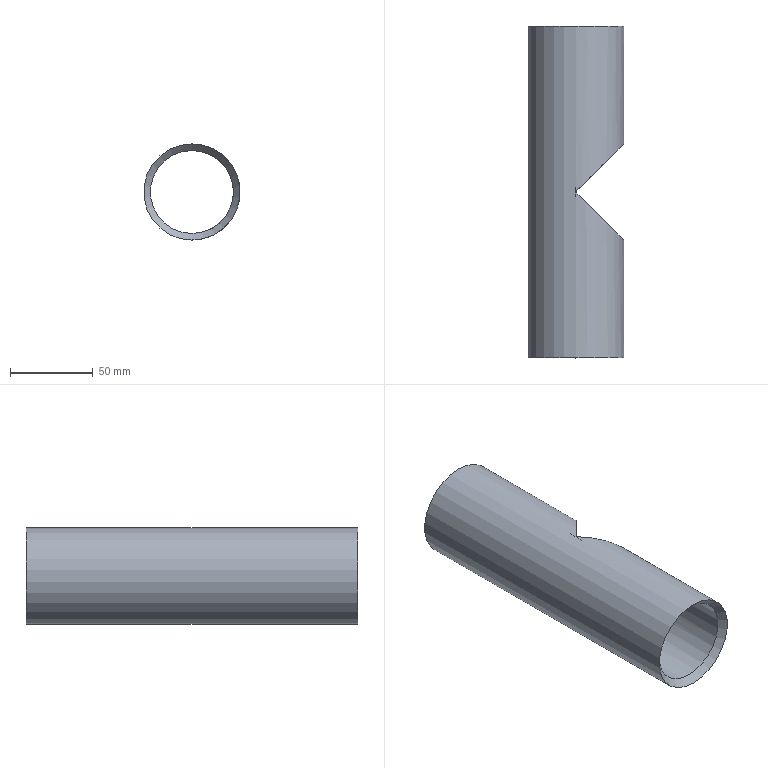Part | STEP file | JBJ-P-1004-01_Default<As Machined> | 1 solid | 8 faces | box 58 x 200 x 58 mm | volume 119017 mm3 | cylinder 4 | plane 2 | cone 2 | commonest cylinder face diameters 58 x3 50 x1
STEP:
#1=CARTESIAN_POINT('',(0.,200.,29.));
#2=VERTEX_POINT('',#1);
#3=CARTESIAN_POINT('',(0.,200.,0.));
#4=DIRECTION('',(0.,1.,0.));
#5=DIRECTION('',(0.,0.,1.));
#6=AXIS2_PLACEMENT_3D('',#3,#4,#5);
#7=CIRCLE('',#6,29.);
#8=EDGE_CURVE('',#2,#2,#7,.T.);
#9=ORIENTED_EDGE('',*,*,#8,.F.);
#10=EDGE_LOOP('',(#9));
#11=FACE_OUTER_BOUND('',#10,.T.);
#12=CARTESIAN_POINT('',(0.,0.,29.));
#13=VERTEX_POINT('',#12);
#14=CARTESIAN_POINT('',(0.,0.,0.));
#15=DIRECTION('',(0.,1.,0.));
#16=DIRECTION('',(0.,0.,1.));
#17=AXIS2_PLACEMENT_3D('',#14,#15,#16);
#18=CIRCLE('',#17,29.);
#19=EDGE_CURVE('',#13,#13,#18,.T.);
#20=ORIENTED_EDGE('',*,*,#19,.T.);
#21=EDGE_LOOP('',(#20));
#22=FACE_OUTER_BOUND('',#21,.T.);
#23=CARTESIAN_POINT('',(0.,100.,-29.));
#24=VERTEX_POINT('',#23);
#25=CARTESIAN_POINT('',(0.,100.,29.));
#26=VERTEX_POINT('',#25);
#27=CARTESIAN_POINT('',(0.,100.,-29.));
#28=CARTESIAN_POINT('',(58.,158.,-29.));
#29=CARTESIAN_POINT('',(58.,158.,29.));
#30=CARTESIAN_POINT('',(0.,100.,29.));
#31=(BOUNDED_CURVE()B_SPLINE_CURVE(3,(#27,#28,#29,#30),.UNSPECIFIED.,.F.,.F.)B_SPLINE_CURVE_WITH_KNOTS((4,4),(1.571,4.712),.UNSPECIFIED.)CURVE()GEOMETRIC_REPRESENTATION_ITEM()RATIONAL_B_SPLINE_CURVE((1.,0.3333,0.3333,1.))REPRESENTATION_ITEM(''));
#32=EDGE_CURVE('',#24,#26,#31,.T.);
#33=ORIENTED_EDGE('',*,*,#32,.F.);
#34=CARTESIAN_POINT('',(0.,100.,29.));
#35=CARTESIAN_POINT('',(58.,42.,29.));
#36=CARTESIAN_POINT('',(58.,42.,-29.));
#37=CARTESIAN_POINT('',(0.,100.,-29.));
#38=(BOUNDED_CURVE()B_SPLINE_CURVE(3,(#34,#35,#36,#37),.UNSPECIFIED.,.F.,.F.)B_SPLINE_CURVE_WITH_KNOTS((4,4),(4.712,7.854),.UNSPECIFIED.)CURVE()GEOMETRIC_REPRESENTATION_ITEM()RATIONAL_B_SPLINE_CURVE((1.,0.3333,0.3333,1.))REPRESENTATION_ITEM(''));
#39=EDGE_CURVE('',#26,#24,#38,.T.);
#40=ORIENTED_EDGE('',*,*,#39,.F.);
#41=EDGE_LOOP('',(#33,#40));
#42=FACE_BOUND('',#41,.T.);
#43=CARTESIAN_POINT('',(0.,200.,0.));
#44=DIRECTION('',(0.,-1.,0.));
#45=DIRECTION('',(0.,0.,-1.));
#46=AXIS2_PLACEMENT_3D('',#43,#44,#45);
#47=CYLINDRICAL_SURFACE('',#46,29.);
#48=ADVANCED_FACE('',(#11,#22,#42),#47,.T.);
#49=CARTESIAN_POINT('',(0.,4.,25.));
#50=VERTEX_POINT('',#49);
#51=CARTESIAN_POINT('',(0.,4.,0.));
#52=DIRECTION('',(0.,-1.,0.));
#53=DIRECTION('',(0.,0.,1.));
#54=AXIS2_PLACEMENT_3D('',#51,#52,#53);
#55=CIRCLE('',#54,25.);
#56=EDGE_CURVE('',#50,#50,#55,.T.);
#57=ORIENTED_EDGE('',*,*,#56,.T.);
#58=EDGE_LOOP('',(#57));
#59=FACE_OUTER_BOUND('',#58,.T.);
#60=CARTESIAN_POINT('',(0.,196.,25.));
#61=VERTEX_POINT('',#60);
#62=CARTESIAN_POINT('',(0.,196.,0.));
#63=DIRECTION('',(0.,1.,0.));
#64=DIRECTION('',(0.,0.,1.));
#65=AXIS2_PLACEMENT_3D('',#62,#63,#64);
#66=CIRCLE('',#65,25.);
#67=EDGE_CURVE('',#61,#61,#66,.T.);
#68=ORIENTED_EDGE('',*,*,#67,.T.);
#69=EDGE_LOOP('',(#68));
#70=FACE_OUTER_BOUND('',#69,.T.);
#71=CARTESIAN_POINT('',(0.,114.697,-25.));
#72=VERTEX_POINT('',#71);
#73=CARTESIAN_POINT('',(0.,114.697,25.));
#74=VERTEX_POINT('',#73);
#75=CARTESIAN_POINT('',(0.,114.697,-25.));
#76=CARTESIAN_POINT('',(0.894,114.697,-25.));
#77=CARTESIAN_POINT('',(1.77,114.779,-24.952));
#78=CARTESIAN_POINT('',(3.061,115.006,-24.816));
#79=CARTESIAN_POINT('',(3.487,115.099,-24.759));
#80=CARTESIAN_POINT('',(4.333,115.317,-24.625));
#81=CARTESIAN_POINT('',(4.754,115.442,-24.548));
#82=CARTESIAN_POINT('',(5.994,115.853,-24.286));
#83=CARTESIAN_POINT('',(6.787,116.174,-24.075));
#84=CARTESIAN_POINT('',(8.322,116.876,-23.588));
#85=CARTESIAN_POINT('',(9.064,117.257,-23.312));
#86=CARTESIAN_POINT('',(10.51,118.058,-22.697));
#87=CARTESIAN_POINT('',(11.215,118.48,-22.357));
#88=CARTESIAN_POINT('',(12.573,119.334,-21.622));
#89=CARTESIAN_POINT('',(13.227,119.767,-21.228));
#90=CARTESIAN_POINT('',(15.125,121.069,-19.964));
#91=CARTESIAN_POINT('',(16.306,121.941,-19.013));
#92=CARTESIAN_POINT('',(17.689,122.997,-17.67));
#93=CARTESIAN_POINT('',(17.961,123.207,-17.394));
#94=CARTESIAN_POINT('',(18.495,123.623,-16.825));
#95=CARTESIAN_POINT('',(18.757,123.829,-16.532));
#96=CARTESIAN_POINT('',(19.524,124.435,-15.635));
#97=CARTESIAN_POINT('',(20.007,124.824,-15.011));
#98=CARTESIAN_POINT('',(21.377,125.937,-13.059));
#99=CARTESIAN_POINT('',(22.184,126.608,-11.649));
#100=CARTESIAN_POINT('',(23.545,127.753,-8.571));
#101=CARTESIAN_POINT('',(24.075,128.206,-6.958));
#102=CARTESIAN_POINT('',(24.531,128.597,-4.838));
#103=CARTESIAN_POINT('',(24.612,128.666,-4.409));
#104=CARTESIAN_POINT('',(24.752,128.786,-3.54));
#105=CARTESIAN_POINT('',(24.811,128.837,-3.101));
#106=CARTESIAN_POINT('',(24.951,128.958,-1.79));
#107=CARTESIAN_POINT('',(24.999,128.999,-0.9146));
#108=CARTESIAN_POINT('',(25.001,129.001,0.8371));
#109=CARTESIAN_POINT('',(24.957,128.963,1.714));
#110=CARTESIAN_POINT('',(24.82,128.845,3.03));
#111=CARTESIAN_POINT('',(24.762,128.795,3.47));
#112=CARTESIAN_POINT('',(24.625,128.677,4.338));
#113=CARTESIAN_POINT('',(24.545,128.609,4.766));
#114=CARTESIAN_POINT('',(24.275,128.377,6.039));
#115=CARTESIAN_POINT('',(24.053,128.187,6.868));
#116=CARTESIAN_POINT('',(23.66,127.853,8.086));
#117=CARTESIAN_POINT('',(23.519,127.733,8.487));
#118=CARTESIAN_POINT('',(23.217,127.478,9.281));
#119=CARTESIAN_POINT('',(23.056,127.342,9.674));
#120=CARTESIAN_POINT('',(22.213,126.632,11.593));
#121=CARTESIAN_POINT('',(21.409,125.962,13.009));
#122=CARTESIAN_POINT('',(20.259,125.028,14.654));
#123=CARTESIAN_POINT('',(20.021,124.836,14.977));
#124=CARTESIAN_POINT('',(19.535,124.446,15.606));
#125=CARTESIAN_POINT('',(19.286,124.247,15.912));
#126=CARTESIAN_POINT('',(18.525,123.644,16.806));
#127=CARTESIAN_POINT('',(17.995,123.232,17.371));
#128=CARTESIAN_POINT('',(16.345,121.97,18.979));
#129=CARTESIAN_POINT('',(15.163,121.096,19.936));
#130=CARTESIAN_POINT('',(13.247,119.781,21.216));
#131=CARTESIAN_POINT('',(12.586,119.343,21.614));
#132=CARTESIAN_POINT('',(11.231,118.489,22.349));
#133=CARTESIAN_POINT('',(10.535,118.073,22.685));
#134=CARTESIAN_POINT('',(9.096,117.274,23.3));
#135=CARTESIAN_POINT('',(8.354,116.891,23.577));
#136=CARTESIAN_POINT('',(6.811,116.184,24.068));
#137=CARTESIAN_POINT('',(6.005,115.858,24.282));
#138=CARTESIAN_POINT('',(4.363,115.311,24.631));
#139=CARTESIAN_POINT('',(3.522,115.089,24.766));
#140=CARTESIAN_POINT('',(2.221,114.858,24.905));
#141=CARTESIAN_POINT('',(1.779,114.798,24.941));
#142=CARTESIAN_POINT('',(0.8921,114.717,24.988));
#143=CARTESIAN_POINT('',(0.4469,114.697,25.));
#144=CARTESIAN_POINT('',(0.,114.697,25.));
#145=B_SPLINE_CURVE_WITH_KNOTS('',3,(#75,#76,#77,#78,#79,#80,#81,#82,#83,#84,#85,#86,#87,#88,#89,#90,#91,#92,#93,#94,#95,#96,#97,#98,#99,#100,#101,#102,#103,#104,#105,#106,#107,#108,#109,#110,#111,#112,#113,#114,#115,#116,#117,#118,#119,#120,#121,#122,#123,#124,#125,#126,#127,#128,#129,#130,#131,#132,#133,#134,#135,#136,#137,#138,#139,#140,#141,#142,#143,#144),.UNSPECIFIED.,.F.,.F.,(4,2,2,2,2,2,2,2,2,2,2,2,2,2,2,2,2,2,2,2,2,2,2,2,2,2,2,2,2,2,2,2,2,2,4),(0.,0.002635,0.003953,0.00527,0.007905,0.01054,0.01318,0.01581,0.02108,0.0224,0.02372,0.02635,0.03162,0.03689,0.03821,0.03953,0.04216,0.0448,0.04611,0.04743,0.05007,0.05138,0.0527,0.05797,0.05929,0.06061,0.06324,0.06851,0.07115,0.07378,0.07642,0.07905,0.08169,0.08301,0.08432),.UNSPECIFIED.);
#146=EDGE_CURVE('',#72,#74,#145,.T.);
#147=ORIENTED_EDGE('',*,*,#146,.T.);
#148=CARTESIAN_POINT('',(0.,85.303,25.));
#149=VERTEX_POINT('',#148);
#150=CARTESIAN_POINT('',(0.,200.,25.));
#151=DIRECTION('',(0.,-1.,0.));
#152=VECTOR('',#151,1000.);
#153=LINE('',#150,#152);
#154=EDGE_CURVE('',#74,#149,#153,.T.);
#155=ORIENTED_EDGE('',*,*,#154,.T.);
#156=CARTESIAN_POINT('',(0.,85.303,-25.));
#157=VERTEX_POINT('',#156);
#158=CARTESIAN_POINT('',(0.,85.303,25.));
#159=CARTESIAN_POINT('',(0.894,85.303,25.));
#160=CARTESIAN_POINT('',(1.77,85.221,24.952));
#161=CARTESIAN_POINT('',(3.061,84.994,24.816));
#162=CARTESIAN_POINT('',(3.487,84.901,24.759));
#163=CARTESIAN_POINT('',(4.333,84.683,24.625));
#164=CARTESIAN_POINT('',(4.754,84.558,24.548));
#165=CARTESIAN_POINT('',(5.994,84.147,24.286));
#166=CARTESIAN_POINT('',(6.787,83.826,24.075));
#167=CARTESIAN_POINT('',(8.322,83.124,23.588));
#168=CARTESIAN_POINT('',(9.064,82.743,23.312));
#169=CARTESIAN_POINT('',(10.51,81.942,22.697));
#170=CARTESIAN_POINT('',(11.215,81.52,22.357));
#171=CARTESIAN_POINT('',(12.573,80.666,21.622));
#172=CARTESIAN_POINT('',(13.227,80.233,21.228));
#173=CARTESIAN_POINT('',(15.125,78.931,19.964));
#174=CARTESIAN_POINT('',(16.306,78.059,19.013));
#175=CARTESIAN_POINT('',(17.689,77.003,17.67));
#176=CARTESIAN_POINT('',(17.961,76.793,17.394));
#177=CARTESIAN_POINT('',(18.495,76.377,16.825));
#178=CARTESIAN_POINT('',(18.757,76.171,16.532));
#179=CARTESIAN_POINT('',(19.524,75.565,15.635));
#180=CARTESIAN_POINT('',(20.007,75.176,15.011));
#181=CARTESIAN_POINT('',(21.377,74.063,13.059));
#182=CARTESIAN_POINT('',(22.184,73.392,11.649));
#183=CARTESIAN_POINT('',(23.545,72.247,8.571));
#184=CARTESIAN_POINT('',(24.075,71.794,6.958));
#185=CARTESIAN_POINT('',(24.531,71.403,4.838));
#186=CARTESIAN_POINT('',(24.612,71.334,4.409));
#187=CARTESIAN_POINT('',(24.752,71.214,3.54));
#188=CARTESIAN_POINT('',(24.811,71.163,3.101));
#189=CARTESIAN_POINT('',(24.951,71.042,1.79));
#190=CARTESIAN_POINT('',(24.999,71.001,0.9146));
#191=CARTESIAN_POINT('',(25.001,70.999,-0.8371));
#192=CARTESIAN_POINT('',(24.957,71.037,-1.714));
#193=CARTESIAN_POINT('',(24.82,71.155,-3.03));
#194=CARTESIAN_POINT('',(24.762,71.205,-3.47));
#195=CARTESIAN_POINT('',(24.625,71.323,-4.338));
#196=CARTESIAN_POINT('',(24.545,71.391,-4.766));
#197=CARTESIAN_POINT('',(24.275,71.623,-6.039));
#198=CARTESIAN_POINT('',(24.053,71.813,-6.868));
#199=CARTESIAN_POINT('',(23.66,72.147,-8.086));
#200=CARTESIAN_POINT('',(23.519,72.267,-8.487));
#201=CARTESIAN_POINT('',(23.217,72.522,-9.281));
#202=CARTESIAN_POINT('',(23.056,72.658,-9.674));
#203=CARTESIAN_POINT('',(22.213,73.368,-11.593));
#204=CARTESIAN_POINT('',(21.409,74.038,-13.009));
#205=CARTESIAN_POINT('',(20.259,74.972,-14.654));
#206=CARTESIAN_POINT('',(20.021,75.164,-14.977));
#207=CARTESIAN_POINT('',(19.535,75.554,-15.606));
#208=CARTESIAN_POINT('',(19.286,75.753,-15.912));
#209=CARTESIAN_POINT('',(18.525,76.356,-16.806));
#210=CARTESIAN_POINT('',(17.995,76.768,-17.371));
#211=CARTESIAN_POINT('',(16.345,78.03,-18.979));
#212=CARTESIAN_POINT('',(15.163,78.904,-19.936));
#213=CARTESIAN_POINT('',(13.247,80.219,-21.216));
#214=CARTESIAN_POINT('',(12.586,80.657,-21.614));
#215=CARTESIAN_POINT('',(11.231,81.511,-22.349));
#216=CARTESIAN_POINT('',(10.535,81.927,-22.685));
#217=CARTESIAN_POINT('',(9.096,82.726,-23.3));
#218=CARTESIAN_POINT('',(8.354,83.109,-23.577));
#219=CARTESIAN_POINT('',(6.811,83.816,-24.068));
#220=CARTESIAN_POINT('',(6.005,84.142,-24.282));
#221=CARTESIAN_POINT('',(4.363,84.689,-24.631));
#222=CARTESIAN_POINT('',(3.522,84.911,-24.766));
#223=CARTESIAN_POINT('',(2.221,85.142,-24.905));
#224=CARTESIAN_POINT('',(1.779,85.202,-24.941));
#225=CARTESIAN_POINT('',(0.8921,85.283,-24.988));
#226=CARTESIAN_POINT('',(0.4469,85.303,-25.));
#227=CARTESIAN_POINT('',(0.,85.303,-25.));
#228=B_SPLINE_CURVE_WITH_KNOTS('',3,(#158,#159,#160,#161,#162,#163,#164,#165,#166,#167,#168,#169,#170,#171,#172,#173,#174,#175,#176,#177,#178,#179,#180,#181,#182,#183,#184,#185,#186,#187,#188,#189,#190,#191,#192,#193,#194,#195,#196,#197,#198,#199,#200,#201,#202,#203,#204,#205,#206,#207,#208,#209,#210,#211,#212,#213,#214,#215,#216,#217,#218,#219,#220,#221,#222,#223,#224,#225,#226,#227),.UNSPECIFIED.,.F.,.F.,(4,2,2,2,2,2,2,2,2,2,2,2,2,2,2,2,2,2,2,2,2,2,2,2,2,2,2,2,2,2,2,2,2,2,4),(0.,0.002635,0.003953,0.00527,0.007905,0.01054,0.01318,0.01581,0.02108,0.0224,0.02372,0.02635,0.03162,0.03689,0.03821,0.03953,0.04216,0.0448,0.04611,0.04743,0.05007,0.05138,0.0527,0.05797,0.05929,0.06061,0.06324,0.06851,0.07115,0.07378,0.07642,0.07905,0.08169,0.08301,0.08432),.UNSPECIFIED.);
#229=EDGE_CURVE('',#149,#157,#228,.T.);
#230=ORIENTED_EDGE('',*,*,#229,.T.);
#231=CARTESIAN_POINT('',(0.,200.,-25.));
#232=DIRECTION('',(0.,1.,0.));
#233=VECTOR('',#232,1000.);
#234=LINE('',#231,#233);
#235=EDGE_CURVE('',#157,#72,#234,.T.);
#236=ORIENTED_EDGE('',*,*,#235,.T.);
#237=EDGE_LOOP('',(#147,#155,#230,#236));
#238=FACE_BOUND('',#237,.T.);
#239=CARTESIAN_POINT('',(0.,200.,0.));
#240=DIRECTION('',(0.,-1.,0.));
#241=DIRECTION('',(0.,0.,-1.));
#242=AXIS2_PLACEMENT_3D('',#239,#240,#241);
#243=CYLINDRICAL_SURFACE('',#242,25.);
#244=ADVANCED_FACE('',(#59,#70,#238),#243,.F.);
#245=ORIENTED_EDGE('',*,*,#39,.T.);
#246=CARTESIAN_POINT('',(0.,100.,0.));
#247=DIRECTION('',(1.,0.,0.));
#248=DIRECTION('',(0.,0.,-1.));
#249=AXIS2_PLACEMENT_3D('',#246,#247,#248);
#250=CIRCLE('',#249,29.);
#251=EDGE_CURVE('',#157,#24,#250,.T.);
#252=ORIENTED_EDGE('',*,*,#251,.F.);
#253=ORIENTED_EDGE('',*,*,#229,.F.);
#254=CARTESIAN_POINT('',(0.,100.,0.));
#255=DIRECTION('',(1.,0.,0.));
#256=DIRECTION('',(0.,0.,-1.));
#257=AXIS2_PLACEMENT_3D('',#254,#255,#256);
#258=CIRCLE('',#257,29.);
#259=EDGE_CURVE('',#26,#149,#258,.T.);
#260=ORIENTED_EDGE('',*,*,#259,.F.);
#261=EDGE_LOOP('',(#245,#252,#253,#260));
#262=FACE_OUTER_BOUND('',#261,.T.);
#263=CARTESIAN_POINT('',(29.,100.,0.));
#264=DIRECTION('',(-1.,0.,0.));
#265=DIRECTION('',(0.,0.,1.));
#266=AXIS2_PLACEMENT_3D('',#263,#264,#265);
#267=CYLINDRICAL_SURFACE('',#266,29.);
#268=ADVANCED_FACE('',(#262),#267,.F.);
#269=CARTESIAN_POINT('',(0.,100.,0.));
#270=DIRECTION('',(1.,0.,0.));
#271=DIRECTION('',(0.,0.,-1.));
#272=AXIS2_PLACEMENT_3D('',#269,#270,#271);
#273=CIRCLE('',#272,29.);
#274=EDGE_CURVE('',#24,#72,#273,.T.);
#275=ORIENTED_EDGE('',*,*,#274,.F.);
#276=ORIENTED_EDGE('',*,*,#32,.T.);
#277=CARTESIAN_POINT('',(0.,100.,0.));
#278=DIRECTION('',(1.,0.,0.));
#279=DIRECTION('',(0.,0.,-1.));
#280=AXIS2_PLACEMENT_3D('',#277,#278,#279);
#281=CIRCLE('',#280,29.);
#282=EDGE_CURVE('',#74,#26,#281,.T.);
#283=ORIENTED_EDGE('',*,*,#282,.F.);
#284=ORIENTED_EDGE('',*,*,#146,.F.);
#285=EDGE_LOOP('',(#275,#276,#283,#284));
#286=FACE_OUTER_BOUND('',#285,.T.);
#287=CARTESIAN_POINT('',(29.,100.,0.));
#288=DIRECTION('',(-1.,0.,0.));
#289=DIRECTION('',(0.,0.,1.));
#290=AXIS2_PLACEMENT_3D('',#287,#288,#289);
#291=CYLINDRICAL_SURFACE('',#290,29.);
#292=ADVANCED_FACE('',(#286),#291,.F.);
#293=ORIENTED_EDGE('',*,*,#282,.T.);
#294=ORIENTED_EDGE('',*,*,#259,.T.);
#295=ORIENTED_EDGE('',*,*,#154,.F.);
#296=EDGE_LOOP('',(#293,#294,#295));
#297=FACE_OUTER_BOUND('',#296,.T.);
#298=CARTESIAN_POINT('',(0.,100.,0.));
#299=DIRECTION('',(1.,0.,0.));
#300=DIRECTION('',(0.,0.,-1.));
#301=AXIS2_PLACEMENT_3D('',#298,#299,#300);
#302=PLANE('',#301);
#303=ADVANCED_FACE('',(#297),#302,.T.);
#304=ORIENTED_EDGE('',*,*,#251,.T.);
#305=ORIENTED_EDGE('',*,*,#274,.T.);
#306=ORIENTED_EDGE('',*,*,#235,.F.);
#307=EDGE_LOOP('',(#304,#305,#306));
#308=FACE_OUTER_BOUND('',#307,.T.);
#309=CARTESIAN_POINT('',(0.,100.,0.));
#310=DIRECTION('',(1.,0.,0.));
#311=DIRECTION('',(0.,0.,-1.));
#312=AXIS2_PLACEMENT_3D('',#309,#310,#311);
#313=PLANE('',#312);
#314=ADVANCED_FACE('',(#308),#313,.T.);
#315=ORIENTED_EDGE('',*,*,#56,.F.);
#316=EDGE_LOOP('',(#315));
#317=FACE_BOUND('',#316,.T.);
#318=ORIENTED_EDGE('',*,*,#19,.F.);
#319=EDGE_LOOP('',(#318));
#320=FACE_OUTER_BOUND('',#319,.T.);
#321=CARTESIAN_POINT('',(0.,0.,0.));
#322=DIRECTION('',(0.,-1.,0.));
#323=DIRECTION('',(0.,0.,-1.));
#324=AXIS2_PLACEMENT_3D('',#321,#322,#323);
#325=CONICAL_SURFACE('',#324,29.,0.7854);
#326=ADVANCED_FACE('',(#317,#320),#325,.F.);
#327=ORIENTED_EDGE('',*,*,#8,.T.);
#328=EDGE_LOOP('',(#327));
#329=FACE_OUTER_BOUND('',#328,.T.);
#330=ORIENTED_EDGE('',*,*,#67,.F.);
#331=EDGE_LOOP('',(#330));
#332=FACE_BOUND('',#331,.T.);
#333=CARTESIAN_POINT('',(0.,196.,0.));
#334=DIRECTION('',(0.,1.,0.));
#335=DIRECTION('',(0.,0.,1.));
#336=AXIS2_PLACEMENT_3D('',#333,#334,#335);
#337=CONICAL_SURFACE('',#336,25.,0.7854);
#338=ADVANCED_FACE('',(#329,#332),#337,.F.);
#339=CLOSED_SHELL('',(#48,#244,#268,#292,#303,#314,#326,#338));
#340=MANIFOLD_SOLID_BREP('',#339);
#341=CARTESIAN_POINT('',(0.,0.,0.));
#342=DIRECTION('',(0.,0.,1.));
#343=DIRECTION('',(1.,0.,0.));
#344=AXIS2_PLACEMENT_3D('',#341,#342,#343);
#345=(LENGTH_UNIT()NAMED_UNIT(*)SI_UNIT(.MILLI.,.METRE.));
#346=UNCERTAINTY_MEASURE_WITH_UNIT(LENGTH_MEASURE(0.00001),#345,'','');
#347=(NAMED_UNIT(*)PLANE_ANGLE_UNIT()SI_UNIT($,.RADIAN.));
#348=(NAMED_UNIT(*)SI_UNIT($,.STERADIAN.)SOLID_ANGLE_UNIT());
#349=(GEOMETRIC_REPRESENTATION_CONTEXT(3)GLOBAL_UNCERTAINTY_ASSIGNED_CONTEXT((#346))GLOBAL_UNIT_ASSIGNED_CONTEXT((#345,#347,#348))REPRESENTATION_CONTEXT('',''));
#350=ADVANCED_BREP_SHAPE_REPRESENTATION('',(#340,#344),#349);